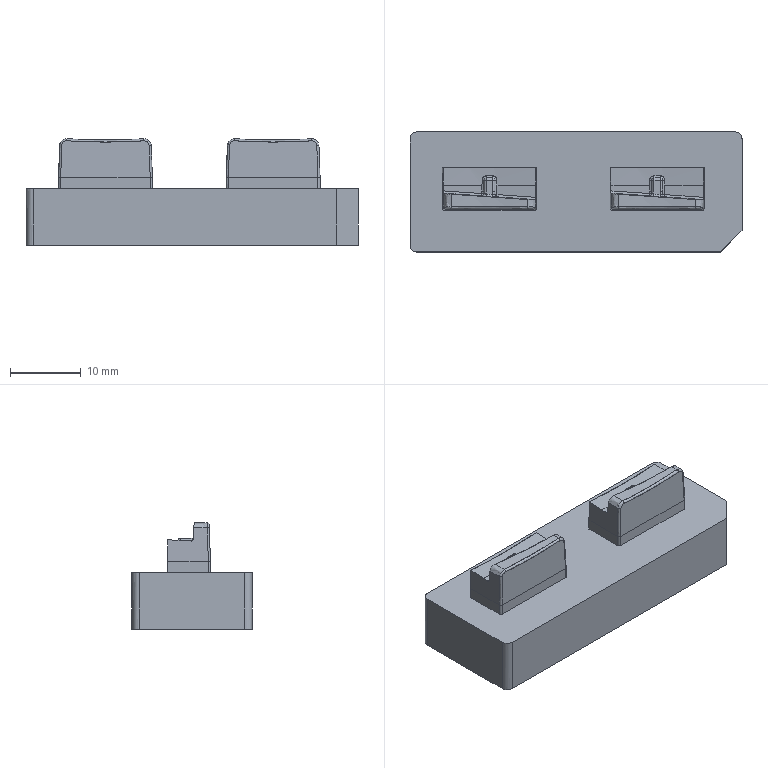NC program | PowerMill | posted with a generic post | part box 47 x 17 x 15.061 mm
Lines 9409 to 10596 of 212044:
N9506 M6
N9507 S22000 M03
N9508 G00 G90 X0.0 Y0.0
N9509 G43 Z9.8009 H27
N9510
N9511 G05 P10000 R4
N9512 X-17.8429 Y1.3228
N9513 Z-1.5208
N9514 G01 Z-2.7208 F1200.0
N9515 X-17.853 Y1.3321 F2000.0
N9516 G03 X-18.0279 Y1.3244 I-0.0836 J-0.0913
N9517 G01 X-18.4675 Y0.8444
N9518 X-18.6964 Y0.72
N9519 X-18.9377 Y0.7308
N9520 X-19.1504 Y0.8766
N9521 X-19.4244 Y0.1186
N9522 X-19.4125 Y0.1119
N9523 G03 X-19.244 Y0.1591 I0.0607 J0.1078
N9524 G01 X-19.1789 Y0.2749
N9525 X-19.0846 Y0.3619
N9526 X-18.9377 Y0.4348
N9527 X-18.6964 Y0.4464
N9528 X-17.1589 Y0.2507
N9529 X-17.0443 Y1.2533 Z-2.7704
N9530 X-17.0545 Y1.2625
N9531 G03 X-17.2293 Y1.2544 I-0.0833 J-0.0914
N9532 G01 X-17.9441 Y0.4701
N9533 X-17.9502 Y0.458
N9534 X-17.9544 Y0.4462
N9535 X-17.9553 Y0.4337
N9536 X-17.9552 Y0.4331
N9537 X-17.9528 Y0.4208
N9538 X-17.9472 Y0.4096
N9539 X-17.9469 Y0.4091
N9540 X-17.9385 Y0.3997
N9541 X-17.928 Y0.3929
N9542 X-17.9158 Y0.3871
N9543 X-17.7315 Y0.3546
N9544 X-16.364 Y0.2017
N9545 G00 Z2.8945
N9546 G01 X-10.9304 Y1.1631 F10000.0
N9547 G00 Z-1.3221
N9548 G01 Z-2.5221 F1200.0
N9549 X-10.9441 F2000.0
N9550 G03 X-11.0679 Y1.0394 I-0.0001 J-0.1238
N9551 G01 X-11.0683 Y-0.1703
N9552 X-11.0652 Y-0.1826
N9553 X-11.0609 Y-0.1935
N9554 X-11.054 Y-0.203
N9555 X-11.0535 Y-0.2036
N9556 X-11.0445 Y-0.2111
N9557 X-11.0339 Y-0.2162
N9558 X-11.0218 Y-0.2202
N9559 X-9.6544 Y-0.3157
N9560 G00 Z2.8502
N9561 G01 X-10.8978 Y1.2816 F10000.0
N9562 G00 Z-1.3718
N9563 G01 Z-2.5718 F1200.0
N9564 X-10.9116 F2000.0
N9565 G03 X-11.0349 Y1.1574 I0.0004 J-0.1238
N9566 G01 X-11.0308 Y-0.1714
N9567 X-11.0277 Y-0.1837
N9568 X-11.0234 Y-0.1946
N9569 X-11.0165 Y-0.2041
N9570 X-11.016 Y-0.2046
N9571 X-11.007 Y-0.2121
N9572 X-10.9964 Y-0.2171
N9573 X-10.9844 Y-0.2211
N9574 X-9.6005 Y-0.3189
N9575 G00 Z2.806
N9576 G01 X-10.8784 Y1.3445 F10000.0
N9577 G00 Z-1.4214
N9578 G01 Z-2.6214 F1200.0
N9579 X-10.8922 F2000.0
N9580 G03 X-11.016 Y1.2208 I-0.0001 J-0.1238
N9581 G01 X-11.0173 Y-0.1704
N9582 X-11.0142 Y-0.1827
N9583 X-11.0099 Y-0.1936
N9584 X-11.003 Y-0.2032
N9585 X-11.0025 Y-0.2037
N9586 X-10.9935 Y-0.2112
N9587 X-10.9829 Y-0.2163
N9588 X-10.9708 Y-0.2203
N9589 X-9.5759 Y-0.3182
N9590 G00 Z2.7618
N9591 G01 X-10.865 Y1.3458 F10000.0
N9592 G00 Z-1.4711
N9593 G01 Z-2.6711 F1200.0
N9594 X-10.8787 F2000.0
N9595 G03 X-11.0026 Y1.2222 I-0.0002 J-0.1238
N9596 G01 X-11.004 Y-0.1699
N9597 X-11.0008 Y-0.1823
N9598 X-10.9965 Y-0.1932
N9599 X-10.9896 Y-0.2027
N9600 X-10.9891 Y-0.2032
N9601 X-10.9801 Y-0.2108
N9602 X-10.9695 Y-0.2158
N9603 X-10.9574 Y-0.2198
N9604 X-9.5573 Y-0.3172
N9605 G00 Z2.7176
N9606 G01 X-10.8399 Y1.3485 F10000.0
N9607 G00 Z-1.5208
N9608 G01 Z-2.7208 F1200.0
N9609 X-10.8537 Y1.3487 F2000.0
N9610 G03 X-10.9787 Y1.2262 I-0.0013 J-0.1238
N9611 G01 X-10.9936 Y-0.1681
N9612 X-10.9905 Y-0.1806
N9613 X-10.9862 Y-0.1916
N9614 X-10.9793 Y-0.2013
N9615 X-10.9788 Y-0.2018
N9616 X-10.9698 Y-0.2094
N9617 X-10.9591 Y-0.2145
N9618 X-10.9468 Y-0.2185
N9619 X-9.5456 Y-0.3101
N9620 G00 Z2.851
N9621 G01 X-10.8323 Y1.3719 F10000.0
N9622 G00 Z-1.5704
N9623 G01 Z-2.7704 F1200.0
N9624 X-10.8461 Y1.372 F2000.0
N9625 G03 X-10.9708 Y1.2491 I-0.0009 J-0.1238
N9626 G01 X-10.9813 Y-0.1611
N9627 X-10.9782 Y-0.1736
N9628 X-10.9739 Y-0.1846
N9629 X-10.967 Y-0.1942
N9630 X-10.9665 Y-0.1947
N9631 X-10.9574 Y-0.2023
N9632 X-10.9468 Y-0.2074
N9633 X-10.9346 Y-0.2114
N9634 X-9.5377 Y-0.3032
N9635 G00 Z2.8075
N9636 G01 X-10.7994 Y1.4057 F10000.0
N9637 G00 Z-1.6201
N9638 G01 Z-2.8201 F1200.0
N9639 X-10.8132 Y1.4059 F2000.0
N9640 G03 X-10.9393 Y1.2846 I-0.0024 J-0.1237
N9641 G01 X-10.9672 Y-0.1505
N9642 X-10.9642 Y-0.1631
N9643 X-10.9599 Y-0.1742
N9644 X-10.953 Y-0.184
N9645 X-10.9525 Y-0.1845
N9646 X-10.9434 Y-0.1922
N9647 X-10.9326 Y-0.1973
N9648 X-10.9203 Y-0.2014
N9649 X-9.4731 Y-0.2911
N9650 G00 Z2.8945
N9651 G01 X4.3292 Y0.1566 F10000.0
N9652 G00 Z-1.5208
N9653 G01 Z-2.7208 F1200.0
N9654 X4.3398 Y0.1478 F2000.0
N9655 G03 X4.514 Y0.1639 I0.0791 J0.0952
N9656 G01 X4.7043 Y0.3928
N9657 X4.9455 Y0.4559
N9658 X6.5958 Y0.2474
N9659 X5.9033 Y1.3286
N9660 X5.8931 Y1.3378
N9661 G03 X5.7183 Y1.3285 I-0.0828 J-0.092
N9662 G01 X5.6692 Y1.2739
N9663 X5.2632 Y0.8444
N9664 X5.1868 Y0.7779
N9665 X4.9455 Y0.7101
N9666 X4.7043 Y0.7813
N9667 X4.6104 Y0.902
N9668 G00 Z2.851
N9669 G01 X6.7059 Y1.2679 F10000.0
N9670 G00 Z-1.5704
N9671 G01 Z-2.7704 F1200.0
N9672 X6.6957 Y1.2771 F2000.0
N9673 G03 X6.5209 Y1.2683 I-0.083 J-0.0918
N9674 G01 X5.7985 Y0.4691
N9675 X5.7924 Y0.4572
N9676 X5.7883 Y0.4455
N9677 X5.7874 Y0.4331
N9678 X5.7875 Y0.4324
N9679 X5.7898 Y0.4202
N9680 X5.7953 Y0.4091
N9681 X5.7957 Y0.4085
N9682 X5.8039 Y0.3992
N9683 X5.8142 Y0.3924
N9684 X5.8263 Y0.3865
N9685 X5.9105 Y0.3705
N9686 X7.3961 Y0.1988
N9687 G00 Z2.8945
N9688 G01 X12.8137 Y1.1625 F10000.0
N9689 G00 Z-1.3221
N9690 G01 Z-2.5221 F1200.0
N9691 X12.8 F2000.0
N9692 G03 X12.6762 Y1.0388 I-0.0001 J-0.1238
N9693 G01 X12.6756 Y-0.1703
N9694 X12.6787 Y-0.1826
N9695 X12.683 Y-0.1935
N9696 X12.6899 Y-0.203
N9697 X12.6904 Y-0.2036
N9698 X12.6994 Y-0.2111
N9699 X12.71 Y-0.2161
N9700 X12.7221 Y-0.2202
N9701 X14.0894 Y-0.3153
N9702 G00 Z2.8502
N9703 G01 X12.8461 Y1.283 F10000.0
N9704 G00 Z-1.3718
N9705 G01 Z-2.5718 F1200.0
N9706 X12.8323 Y1.2829 F2000.0
N9707 G03 X12.709 Y1.1588 I0.0004 J-0.1237
N9708 G01 X12.7131 Y-0.1711
N9709 X12.7163 Y-0.1834
N9710 X12.7206 Y-0.1943
N9711 X12.7274 Y-0.2038
N9712 X12.7279 Y-0.2043
N9713 X12.7369 Y-0.2118
N9714 X12.7475 Y-0.2168
N9715 X12.7596 Y-0.2208
N9716 X14.1411 Y-0.3176
N9717 G00 Z2.806
N9718 G01 X12.8654 Y1.3421 F10000.0
N9719 G00 Z-1.4214
N9720 G01 Z-2.6214 F1200.0
N9721 X12.8517 F2000.0
N9722 G03 X12.7278 Y1.2184 I-0.0001 J-0.1238
N9723 G01 X12.7266 Y-0.1705
N9724 X12.7298 Y-0.1829
N9725 X12.7341 Y-0.1939
N9726 X12.741 Y-0.2034
N9727 X12.7415 Y-0.2039
N9728 X12.7505 Y-0.2114
N9729 X12.7611 Y-0.2165
N9730 X12.7733 Y-0.2205
N9731 X14.1606 Y-0.313
N9732 G00 Z2.7618
N9733 G01 X12.882 Y1.3435 F10000.0
N9734 G00 Z-1.4711
N9735 G01 Z-2.6711 F1200.0
N9736 X12.8682 Y1.3433 F2000.0
N9737 G03 X12.7456 Y1.2185 I0.0012 J-0.1237
N9738 G01 X12.7468 Y1.0856
N9739 X12.7402 Y-0.1689
N9740 X12.7433 Y-0.1813
N9741 X12.7476 Y-0.1923
N9742 X12.7545 Y-0.2019
N9743 X12.755 Y-0.2024
N9744 X12.7641 Y-0.21
N9745 X12.7748 Y-0.215
N9746 X12.787 Y-0.219
N9747 X14.1734 Y-0.3086
N9748 G00 Z2.7176
N9749 G01 X12.8994 Y1.3498 F10000.0
N9750 G00 Z-1.5208
N9751 G01 Z-2.7208 F1200.0
N9752 X12.8857 Y1.3497 F2000.0
N9753 G03 X12.7627 Y1.2252 I0.0008 J-0.1237
N9754 G01 X12.7637 Y1.0856
N9755 X12.7503 Y-0.1681
N9756 X12.7534 Y-0.1806
N9757 X12.7577 Y-0.1916
N9758 X12.7645 Y-0.2012
N9759 X12.765 Y-0.2018
N9760 X12.774 Y-0.2094
N9761 X12.7847 Y-0.2145
N9762 X12.7969 Y-0.2185
N9763 X13.0255 Y-0.2345
N9764 X14.1991 Y-0.3103
N9765 G00 Z2.851
N9766 G01 X12.9125 Y1.3702 F10000.0
N9767 G00 Z-1.5704
N9768 G01 Z-2.7704 F1200.0
N9769 X12.8988 Y1.3703 F2000.0
N9770 G03 X12.774 Y1.2475 I-0.001 J-0.1238
N9771 G01 X12.7626 Y-0.1618
N9772 X12.7657 Y-0.1743
N9773 X12.77 Y-0.1854
N9774 X12.7769 Y-0.195
N9775 X12.7774 Y-0.1955
N9776 X12.7865 Y-0.2031
N9777 X12.7972 Y-0.2081
N9778 X12.8095 Y-0.2121
N9779 X14.2037 Y-0.3012
N9780 G00 Z2.8075
N9781 G01 X12.9445 Y1.4055 F10000.0
N9782 G00 Z-1.6201
N9783 G01 Z-2.8201 F1200.0
N9784 X12.9308 Y1.4058 F2000.0
N9785 G03 X12.8046 Y1.2845 I-0.0025 J-0.1237
N9786 G01 X12.7767 Y-0.1507
N9787 X12.7797 Y-0.1633
N9788 X12.784 Y-0.1744
N9789 X12.7909 Y-0.1842
N9790 X12.7913 Y-0.1847
N9791 X12.8005 Y-0.1924
N9792 X12.8112 Y-0.1975
N9793 X12.8235 Y-0.2016
N9794 X14.2773 Y-0.2953
N9795 G00 Z2.851
N9796 G01 X18.5929 Y-0.0413 F10000.0
N9797 G00 Z-1.5704
N9798 G01 Z-2.7704 F1200.0
N9799 X18.5828 Y-0.0319 F2000.0
N9800 G03 X18.4079 Y-0.0378 I-0.0845 J-0.0904
N9801 G01 X18.3304 Y-0.1206
N9802 X18.214 Y-0.1908
N9803 X17.9727 Y-0.2239
N9804 X17.7458 Y-0.1206
N9805 X17.4902 Y0.1221
N9806 X16.9632 Y0.6963
N9807 X15.7018 Y-0.2627
N9808 X15.7014 Y-0.2764
N9809 G03 X15.8215 Y-0.4038 I0.1237 J-0.0037
N9810 G01 X17.7315 Y-0.4598
N9811 X17.9727 Y-0.3921
N9812 X18.214 Y-0.4275
N9813 X18.4345 Y-0.6031
N9814 X18.4581 Y-0.6682
N9815 G00 Z2.8075
N9816 G01 X14.8066 Y-0.1868 F10000.0
N9817 G00 Z-1.6201
N9818 G01 Z-2.8201 F1200.0
N9819 X14.806 Y-0.2005 F2000.0
N9820 G03 X14.9246 Y-0.3292 I0.1237 J-0.005
N9821 G01 X16.7665 Y-0.4041
N9822 X16.9962 Y-0.3993
N9823 X17.0099 Y-0.395
N9824 X17.0219 Y-0.3892
N9825 X17.0318 Y-0.3802
N9826 X17.0322 Y-0.3798
N9827 X17.0392 Y-0.3684
N9828 X17.0427 Y-0.3555
N9829 X17.0428 Y-0.355
N9830 X17.0425 Y-0.3416
N9831 X17.0385 Y-0.3289
N9832 X17.0324 Y-0.3159
N9833 X16.2082 Y0.6031
N9834 X16.0457 Y0.7548
N9835 G00 Z5.6437
N9836 G01 X13.8538 Y-0.1772 F10000.0
N9837 G00 Z-2.7197
N9838 G01 X13.8919 Y0.0388 Z-2.7236 F1200.0
N9839 X14.0569 Y0.3246 Z-2.7293
N9840 X14.3096 Y0.5366 Z-2.7351
N9841 X14.6197 Y0.6495 Z-2.7408
N9842 X14.9496 Z-2.7466
N9843 X15.2596 Y0.5366 Z-2.7523
N9844 X15.5124 Y0.3246 Z-2.7581
N9845 X15.6773 Y0.0388 Z-2.7639
N9846 X15.7346 Y-0.2861 Z-2.7696
N9847 X15.7335 Y-0.2923 Z-2.7697
N9848 X15.3201 Y-0.2844 Z-2.7769
N9849 X14.7862 Y-0.2561 Z-2.7863
N9850 X13.8487 Y-0.2065 Z-2.8027
N9851 X13.8919 Y0.0388 Z-2.807
N9852 X14.0569 Y0.3246 Z-2.8128
N9853 X14.3096 Y0.5366 Z-2.8185
N9854 X14.6197 Y0.6495 Z-2.8243
N9855 X14.9496 Z-2.83
N9856 X15.2596 Y0.5366 Z-2.8358
N9857 X15.5124 Y0.3246 Z-2.8416
N9858 X15.6773 Y0.0388 Z-2.8473
N9859 X15.7346 Y-0.2861 Z-2.8531
N9860 X15.7335 Y-0.2923 Z-2.8532
N9861 X15.3201 Y-0.2844 Z-2.8604
N9862 X14.7862 Y-0.2561 Z-2.8697
N9863 X14.7846 Y-0.2861
N9864 X14.8163 Y0.1739 F2000.0
N9865 G03 X14.8937 Y0.4082 I0.0087 J0.127
N9866 G01 X13.5722 Y1.254
N9867 G03 X13.3028 Y1.1079 I-0.0944 J-0.1475
N9868 G01 X13.2979 Y0.4665
N9869 G03 X13.4842 Y0.2655 I0.2 J-0.0015
N9870 G01 X14.8163 Y0.1739
N9871 X14.7846 Y-0.2861
N9872 X15.319 Y-0.3144
N9873 X16.0774 Y-0.3288
N9874 X16.1238 Y-0.2997
N9875 X16.1156 Y-0.2455
N9876 X16.0039 Y-0.1206
N9877 X15.0778 Y0.8977
N9878 X14.8298 Y1.0856
N9879 X14.4099 Y1.3268
N9880 X14.361 Y1.3848
N9881 X14.3533 Y1.3921
N9882 X14.3443 Y1.3977
N9883 X13.1478 Y1.9692
N9884 X12.8826 Y2.0517
N9885 X12.833 Y2.0399
N9886 X12.8196 Y1.9906
N9887 X12.8696 Y1.8093
N9888 X12.7912 Y-0.1311
N9889 X12.8042 Y-0.1668
N9890 X12.8385 Y-0.1831
N9891 X14.7846 Y-0.2861
N9892 G00 Z5.6388
N9893 G01 X13.5404 Y-0.1549 F10000.0
N9894 G00 Z-2.7694
N9895 G01 X12.8888 Y-0.1203 Z-2.7808 F1200.0
N9896 X12.8699 Y-0.0991 Z-2.7813
N9897 X12.8959 Y0.3287 Z-2.7888
N9898 X12.9403 Y1.0568 Z-2.8015
N9899 X12.9694 Y1.0733 Z-2.8021
N9900 X13.7507 Y0.6692 Z-2.8174
N9901 X13.7587 Y0.6554 Z-2.8177
N9902 X13.816 Y0.3305 Z-2.8235
N9903 X13.7587 Y0.0056 Z-2.8292
N9904 X13.6623 Y-0.1614 Z-2.8326
N9905 X12.8888 Y-0.1203 Z-2.8461
N9906 X12.8699 Y-0.0991 Z-2.8466
N9907 X12.8959 Y0.3287 Z-2.8541
N9908 X12.9403 Y1.0568 Z-2.8668
N9909 X12.9694 Y1.0733 Z-2.8674
N9910 X13.7507 Y0.6692 Z-2.8827
N9911 X13.7587 Y0.6554 Z-2.883
N9912 X13.816 Y0.3305 Z-2.8888
N9913 X13.7587 Y0.0056 Z-2.8945
N9914 X13.6623 Y-0.1614 Z-2.8979
N9915 X12.8888 Y-0.1203 Z-2.9114
N9916 X12.8699 Y-0.0991 Z-2.9119
N9917 X12.8959 Y0.3287 Z-2.9194
N9918 X12.866 Y0.3305
N9919 X13.3659 F2000.0
N9920 X13.3701 Y0.3263
N9921 X13.3743 Y0.3305
N9922 X13.3701 Y0.3347
N9923 X13.3659 Y0.3305
N9924 X12.866
N9925 X12.8399 Y-0.0973
N9926 X12.8525 Y-0.1336
N9927 X12.8872 Y-0.1503
N9928 X14.5953 Y-0.2409
N9929 X15.155 Y-0.2516
N9930 X15.2014 Y-0.2226
N9931 X15.1934 Y-0.1685
N9932 X15.1511 Y-0.1206
N9933 X14.9732 Y0.0707
N9934 X12.9832 Y1.1
N9935 X12.9356 Y1.099
N9936 X12.9103 Y1.0586
N9937 X12.866 Y0.3305
N9938 X13.0254 Y0.1081 Z-2.819
N9939 X12.9687 Y0.1379 Z-2.8202 F1200.0
N9940 X12.9513 Y0.1385 Z-2.8205
N9941 X12.9395 Y0.122 Z-2.8208
N9942 X12.9237 Y-0.051 Z-2.8238
N9943 X12.9427 Y-0.0728 Z-2.8244
N9944 X13.3195 Y-0.0892 Z-2.8309
N9945 X13.3297 Y-0.0515 Z-2.8316
N9946 X12.9687 Y0.1379 Z-2.8387
N9947 X12.9513 Y0.1385 Z-2.839
N9948 X12.9395 Y0.122 Z-2.8394
N9949 X12.9237 Y-0.051 Z-2.8424
N9950 X12.9427 Y-0.0728 Z-2.8429
N9951 X13.3195 Y-0.0892 Z-2.8495
N9952 X13.3297 Y-0.0515 Z-2.8502
N9953 X12.9687 Y0.1379 Z-2.8573
N9954 X12.9513 Y0.1385 Z-2.8576
N9955 X12.9395 Y0.122 Z-2.858
N9956 X12.9237 Y-0.051 Z-2.861
N9957 X12.9427 Y-0.0728 Z-2.8615
N9958 X13.3195 Y-0.0892 Z-2.8681
N9959 X13.3297 Y-0.0515 Z-2.8688
N9960 X12.9687 Y0.1379 Z-2.8759
N9961 X12.9513 Y0.1385 Z-2.8762
N9962 X12.9395 Y0.122 Z-2.8765
N9963 X12.9237 Y-0.051 Z-2.8796
N9964 X12.9427 Y-0.0728 Z-2.8801
N9965 X13.3195 Y-0.0892 Z-2.8867
N9966 X13.3297 Y-0.0515 Z-2.8873
N9967 X12.9687 Y0.1379 Z-2.8944
N9968 X12.9513 Y0.1385 Z-2.8948
N9969 X12.9395 Y0.122 Z-2.8951
N9970 X12.9237 Y-0.051 Z-2.8981
N9971 X12.9427 Y-0.0728 Z-2.8986
N9972 X13.3195 Y-0.0892 Z-2.9052
N9973 X13.3297 Y-0.0515 Z-2.9059
N9974 X12.9687 Y0.1379 Z-2.913
N9975 X12.9513 Y0.1385 Z-2.9133
N9976 X12.9395 Y0.122 Z-2.9137
N9977 X12.9237 Y-0.051 Z-2.9167
N9978 X12.9427 Y-0.0728 Z-2.9172
N9979 X13.3195 Y-0.0892 Z-2.9238
N9980 X13.3297 Y-0.0515 Z-2.9245
N9981 X12.9687 Y0.1379 Z-2.9316
N9982 X12.9513 Y0.1385 Z-2.9319
N9983 X12.9395 Y0.122 Z-2.9322
N9984 X12.9237 Y-0.051 Z-2.9353
N9985 X12.9427 Y-0.0728 Z-2.9358
N9986 X13.3195 Y-0.0892 Z-2.9424
N9987 X13.3297 Y-0.0515 Z-2.943
N9988 X12.9687 Y0.1379 Z-2.9502
N9989 X12.9513 Y0.1385 Z-2.9505
N9990 X12.9395 Y0.122 Z-2.9508
N9991 X12.9237 Y-0.051 Z-2.9539
N9992 X12.9427 Y-0.0728 Z-2.9544
N9993 X13.3195 Y-0.0892 Z-2.9609
N9994 X13.3297 Y-0.0515 Z-2.9616
N9995 X12.9687 Y0.1379 Z-2.9687
N9996 X12.9513 Y0.1385 Z-2.969
N9997 X12.9391 Y0.1659
N9998 X12.9188 Y0.1493 F2000.0
N9999 X12.9097 Y0.1248
N10000 X12.8938 Y-0.0482
N10001 X12.9059 Y-0.0857
N10002 X12.9414 Y-0.1028
N10003 X13.3182 Y-0.1192
N10004 X13.3687 Y-0.0822
N10005 X13.3436 Y-0.0249
N10006 X12.9827 Y0.1645
N10007 X12.9611 Y0.1702
N10008 X12.9391 Y0.1659
N10009 G00 Z2.7207
N10010 G01 X8.5418 Y0.2113 F10000.0
N10011 G00 Z-1.3221
N10012 G01 Z-2.5221 F1200.0
N10013 X8.5408 Y0.1976 F2000.0
N10014 G03 X8.6555 Y0.0654 I0.1234 J-0.0088
N10015 G01 X10.2462 Y-0.0475
N10016 X10.2598 Y-0.0447
N10017 X10.2719 Y-0.0404
N10018 X10.2824 Y-0.033
N10019 X10.2829 Y-0.0325
N10020 X10.291 Y-0.0226
N10021 X10.296 Y-0.0108
N10022 X10.2997 Y0.0026
N10023 X10.2939 Y1.4164
N10024 G00 Z2.8502
N10025 G01 X8.4998 Y0.2195 F10000.0
N10026 G00 Z-1.3718
N10027 G01 Z-2.5718 F1200.0
N10028 X8.4988 Y0.2058 F2000.0
N10029 G03 X8.6132 Y0.0734 I0.1234 J-0.009
N10030 G01 X10.2086 Y-0.043
N10031 X10.2222 Y-0.0402
N10032 X10.2343 Y-0.036
N10033 X10.2448 Y-0.0286
N10034 X10.2453 Y-0.0282
N10035 X10.2534 Y-0.0182
N10036 X10.2585 Y-0.0065
N10037 X10.2623 Y0.0069
N10038 X10.2619 Y1.5318
N10039 G00 Z2.806
N10040 G01 X8.4744 Y0.2258 F10000.0
N10041 G00 Z-1.4214
N10042 G01 Z-2.6214 F1200.0
N10043 X8.4734 Y0.2121 F2000.0
N10044 G03 X8.5876 Y0.0795 I0.1234 J-0.0092
N10045 G01 X10.1952 Y-0.0402
N10046 X10.2088 Y-0.0375
N10047 X10.2209 Y-0.0332
N10048 X10.2315 Y-0.0258
N10049 X10.2319 Y-0.0254
N10050 X10.2401 Y-0.0154
N10051 X10.2452 Y-0.0036
N10052 X10.2489 Y0.0097
N10053 X10.2449 Y1.5681
N10054 X10.2461 Y1.5952
N10055 G00 Z2.7618
N10056 G01 X8.4548 Y0.2282 F10000.0
N10057 G00 Z-1.4711
N10058 G01 Z-2.6711 F1200.0
N10059 X8.4537 Y0.2145 F2000.0
N10060 G03 X8.5669 Y0.081 I0.1233 J-0.0102
N10061 G01 X9.3808 Y0.0186
N10062 X10.1953 Y-0.035
N10063 X10.2074 Y-0.0307
N10064 X10.2179 Y-0.0232
N10065 X10.2184 Y-0.0228
N10066 X10.2265 Y-0.0128
N10067 X10.2316 Y-0.001
N10068 X10.2353 Y0.0123
N10069 X10.2278 Y1.5681
N10070 X10.2296 Y1.6063
N10071 G00 Z2.8945
N10072 G01 X8.4484 Y0.2381 F10000.0
N10073 G00 Z-1.5208
N10074 G01 Z-2.7208 F1200.0
N10075 X8.4473 Y0.2244 F2000.0
N10076 G03 X8.561 Y0.0914 I0.1234 J-0.0096
N10077 G01 X10.1696 Y-0.0348
N10078 X10.1833 Y-0.032
N10079 X10.1956 Y-0.0277
N10080 X10.2061 Y-0.0203
N10081 X10.2066 Y-0.0199
N10082 X10.2148 Y-0.0098
N10083 X10.2199 Y0.0021
N10084 X10.2236 Y0.0156
N10085 X10.2088 Y1.5681
N10086 X10.2104 Y1.6046
N10087 G00 Z2.851
N10088 G01 X8.3713 Y0.253 F10000.0
N10089 G00 Z-1.5704
N10090 G01 Z-2.7704 F1200.0
N10091 X8.3702 Y0.2393 F2000.0
N10092 G03 X8.484 Y0.1063 I0.1234 J-0.0097
N10093 G01 X10.1554 Y-0.0243
N10094 X10.1691 Y-0.0215
N10095 X10.1814 Y-0.0172
N10096 X10.192 Y-0.0097
N10097 X10.1924 Y-0.0093
N10098 X10.2006 Y0.0008
N10099 X10.2057 Y0.0127
N10100 X10.2093 Y0.0262
N10101 X10.1898 Y1.5681
N10102 X10.1933 Y1.6561
N10103 X9.3035 Y2.2713 Z-2.8201
N10104 X9.3158 Y2.1344
N10105 G02 X8.682 Y2.2336 I-0.1183 J1.3186
N10106 G01 X8.5962 Y2.2735
N10107 X8.5642 Y2.2636
N10108 X8.2159 Y2.0506
N10109 X8.0966 Y2.0078
N10110 X8.0768 Y1.9947
N10111 X8.0153 Y1.9625
N10112 X7.3671 Y1.2524
N10113 X7.6834 Y0.9117
N10114 X8.3172 Y1.5
N10115 X8.3409 Y1.5188
N10116 X8.5699 Y1.651
N10117 X8.6196 Y1.6712
N10118 X8.6729 Y1.6775
N10119 X8.8571 Y1.6746
N10120 X8.8446 Y1.2139
N10121 X9.1221 Y1.2064
N10122 X9.1699 Y1.1845
N10123 X9.1871 Y1.1349
N10124 X9.1835 Y1.0821
N10125 X9.1628 Y1.0399
N10126 X9.1186 Y1.0243
N10127 X8.8193 Y1.039
N10128 G02 X8.7809 Y1.1906 I0.004 J0.0817
N10129 G01 X8.8 Y1.2021
N10130 X8.8214 Y1.2112
N10131 X8.8446 Y1.2139
N10132 X8.8571 Y1.6746
N10133 X9.2241 Y1.6689
N10134 X9.4927 Y1.6808
N10135 G02 X9.7022 Y1.4828 I0.0095 J-0.1998
N10136 G01 X9.709 Y0.7242
N10137 G02 X9.4932 Y0.523 I-0.2 J-0.0018
N10138 G01 X7.7708 Y0.6601
N10139 G02 X7.6834 Y0.9117 I0.0115 J0.145
N10140 G01 X7.3671 Y1.2524
N10141 X6.6024 Y0.4145
N10142 X6.5962 Y0.4022
N10143 X6.5921 Y0.39
N10144 X6.5914 Y0.3772
N10145 Y0.3765
N10146 X6.5942 Y0.364
N10147 X6.6003 Y0.3527
N10148 X6.6007 Y0.3522
N10149 X6.6096 Y0.343
N10150 X6.6207 Y0.3365
N10151 X6.6335 Y0.3312
N10152 X7.8404 Y0.1875
N10153 X10.142 Y-0.011
N10154 X10.1558 Y-0.0083
N10155 X10.1681 Y-0.004
N10156 X10.1788 Y0.0035
N10157 X10.1793 Y0.0039
N10158 X10.1875 Y0.014
N10159 X10.1926 Y0.026
N10160 X10.1963 Y0.0396
N10161 X10.1837 Y0.9246
N10162 X10.1613 Y1.8093
N10163 X10.2315 Y2.0506
N10164 X10.3955 Y2.2918
N10165 X10.4584 Y2.3515
N10166 X9.6381 Y1.8419 Z-2.7197
N10167 X9.6569 Y1.8512 Z-2.7201 F1200.0
N10168 X9.7036 Y1.7705 Z-2.7217
N10169 X9.7608 Y1.4456 Z-2.7275
N10170 X9.7036 Y1.1207 Z-2.7332
N10171 X9.5386 Y0.8349 Z-2.739
N10172 X9.2859 Y0.6229 Z-2.7448
N10173 X8.9758 Y0.51 Z-2.7505
N10174 X8.6459 Z-2.7563
N10175 X8.3358 Y0.6229 Z-2.762
N10176 X8.0831 Y0.8349 Z-2.7678
N10177 X8.0087 Y0.9638 Z-2.7704
N10178 X8.0352 Y0.9924 Z-2.7711
N10179 X8.8251 Y1.4192 Z-2.7867
N10180 X9.3017 Y1.6767 Z-2.7962
N10181 X9.6569 Y1.8512 Z-2.8031
N10182 X9.7036 Y1.7705 Z-2.8047
N10183 X9.7608 Y1.4456 Z-2.8105
N10184 X9.7036 Y1.1207 Z-2.8162
N10185 X9.5386 Y0.8349 Z-2.822
N10186 X9.2859 Y0.6229 Z-2.8278
N10187 X8.9758 Y0.51 Z-2.8335
N10188 X8.6459 Z-2.8393
N10189 X8.3358 Y0.6229 Z-2.845
N10190 X8.0831 Y0.8349 Z-2.8508
N10191 X8.0087 Y0.9638 Z-2.8534
N10192 X8.0352 Y0.9924 Z-2.8541
N10193 X8.8251 Y1.4192 Z-2.8697
N10194 X8.8109 Y1.4456
N10195 X9.0297 Y1.0371 F2000.0
N10196 X8.6334 Y0.8249
N10197 G03 X8.6767 Y0.616 I0.0525 J-0.0981
N10198 G01 X9.4608 Y0.5507
N10199 G03 X9.6774 Y0.7524 I0.0166 J0.1993
N10200 G01 X9.6732 Y1.1033
N10201 G03 X9.4259 Y1.2494 I-0.168 J-0.002
N10202 G01 X9.0297 Y1.0371
N10203 X8.8109 Y1.4456
N10204 X8.0166 Y1.0164
N10205 X7.4124 Y0.366
N10206 X7.4017 Y0.3157
N10207 X7.441 Y0.2826
N10208 X7.5992 Y0.2569
N10209 X10.1224 Y0.0136
N10210 X10.1616 Y0.0271
N10211 X10.1772 Y0.0655
N10212 X10.1747 Y0.1206
N10213 X10.1058 Y1.8093
N10214 X10.1685 Y2.0506
N10215 X10.1758 Y2.0644
N10216 X10.1665 Y2.1236
N10217 X10.107 Y2.1313
N10218 X9.7704 Y1.9404
N10219 X9.2879 Y1.7034
N10220 X8.8109 Y1.4456
N10221 X9.2649 Y0.6947 Z-2.7694
N10222 X9.2112 Y0.6671 Z-2.7704 F1200.0
N10223 X8.4738 Y0.2878 Z-2.7849
N10224 X8.4803 Y0.2502 Z-2.7856
N10225 X9.05 Y0.1735 Z-2.7956
N10226 X9.9327 Y0.0961 Z-2.8111
N10227 X10.0802 Y0.3516 Z-2.8162
N10228 X10.04 Y1.0617 Z-2.8286
N10229 X10.0108 Y1.0783 Z-2.8292
N10230 X9.2112 Y0.6671 Z-2.8449
N10231 X8.4738 Y0.2878 Z-2.8594
N10232 X8.4803 Y0.2502 Z-2.8601
N10233 X9.05 Y0.1735 Z-2.8701
N10234 X9.9327 Y0.0961 Z-2.8856
N10235 X10.0802 Y0.3516 Z-2.8907
N10236 X10.04 Y1.0617 Z-2.9031
N10237 X10.0108 Y1.0783 Z-2.9037
N10238 X9.2112 Y0.6671 Z-2.9194
N10239 X9.1975 Y0.6938
N10240 X8.4601 Y0.3145 F2000.0
N10241 G03 X8.4763 Y0.2205 I0.0228 J-0.0445
N10242 G01 X9.0467 Y0.1437
N10243 X10.07 Y0.0539
N10244 X10.1093 Y0.068
N10245 X10.1243 Y0.107
N10246 X10.1234 Y0.1206
N10247 X10.0699 Y1.0634
N10248 X10.0448 Y1.1039
N10249 X9.9971 Y1.105
N10250 X9.1975 Y0.6938
N10251 G00 Z2.851
N10252 G01 X-5.1622 Y-0.0004 F10000.0
N10253 G00 Z-1.5704
N10254 G01 Z-2.7704 F1200.0
N10255 X-5.1734 Y0.0076 F2000.0
N10256 G03 X-5.346 Y-0.0209 I-0.072 J-0.1006
N10257 G01 X-5.428 Y-0.1353
N10258 X-5.6692 Y-0.2247
N10259 X-5.9105 Y-0.1877
N10260 X-6.0156 Y-0.1206
N10261 X-6.7796 Y0.6989
N10262 X-8.0198 Y-0.2494
N10263 X-8.0203 Y-0.2632
N10264 G03 X-7.9017 Y-0.3918 I0.1236 J-0.005
N10265 G01 X-6.1278 Y-0.4633
N10266 X-5.6692 Y-0.3917
N10267 X-5.428 Y-0.4841
N10268 X-5.3092 Y-0.6031
N10269 X-5.2877 Y-0.6627
N10270 G00 Z2.8075
N10271 G01 X-8.9278 Y-0.1871 F10000.0
N10272 G00 Z-1.6201
N10273 G01 Z-2.8201 F1200.0
N10274 X-8.9287 Y-0.2008 F2000.0
N10275 G03 X-8.8128 Y-0.332 I0.1235 J-0.0077
N10276 G01 X-8.8054 Y-0.3324
N10277 X-6.7569 Y-0.3935
N10278 X-6.7427 Y-0.3897
N10279 X-6.7302 Y-0.3843
N10280 X-6.7197 Y-0.3755
N10281 X-6.7193 Y-0.3751
N10282 X-6.7119 Y-0.3636
N10283 X-6.708 Y-0.3505
N10284 X-6.7079 Y-0.35
N10285 X-6.708 Y-0.3363
N10286 X-6.712 Y-0.3232
N10287 X-6.7183 Y-0.31
N10288 X-7.6895 Y0.7613
N10289 G00 Z5.6396
N10290 G01 X-9.8977 Y-0.1589 F10000.0
N10291 G00 Z-2.7197
N10292 G01 X-9.8616 Y0.0458 Z-2.7234 F1200.0
N10293 X-9.6967 Y0.3315 Z-2.7291
N10294 X-9.4439 Y0.5436 Z-2.7349
N10295 X-9.1339 Y0.6564 Z-2.7406
N10296 X-8.8039 Z-2.7464
N10297 X-8.4939 Y0.5436 Z-2.7521
N10298 X-8.2412 Y0.3315 Z-2.7579
N10299 X-8.0762 Y0.0458 Z-2.7637
N10300 X-8.0189 Y-0.2792 Z-2.7694
N10301 X-8.0197 Y-0.2838 Z-2.7695
N10302 X-8.9678 Y-0.2492 Z-2.7861
N10303 X-9.769 Y-0.2199 Z-2.8
N10304 X-9.907 Y-0.2118 Z-2.8025
N10305 X-9.8616 Y0.0458 Z-2.807
N10306 X-9.6967 Y0.3315 Z-2.8128
N10307 X-9.4439 Y0.5436 Z-2.8185
N10308 X-9.1339 Y0.6564 Z-2.8243
N10309 X-8.8039 Z-2.8301
N10310 X-8.4939 Y0.5436 Z-2.8358
N10311 X-8.2412 Y0.3315 Z-2.8416
N10312 X-8.0762 Y0.0458 Z-2.8473
N10313 X-8.0189 Y-0.2792 Z-2.8531
N10314 X-8.0197 Y-0.2838 Z-2.8532
N10315 X-8.9678 Y-0.2492 Z-2.8697
N10316 X-8.9689 Y-0.2792
N10317 X-8.9403 Y0.1787 F2000.0
N10318 G03 X-8.8585 Y0.4146 I0.0081 J0.1293
N10319 G01 X-9.1506 Y0.6163
N10320 X-10.1733 Y1.2613
N10321 G03 X-10.4409 Y1.1149 I-0.0931 J-0.1476
N10322 G01 X-10.4453 Y0.4621
N10323 G03 X-10.2577 Y0.2611 I0.2 J-0.0014
N10324 G01 X-8.9403 Y0.1787
N10325 X-8.9689 Y-0.2792
N10326 X-7.6658 Y-0.3268
N10327 G03 X-7.6262 Y-0.2441 I0.0018 J0.05
N10328 G01 X-7.7331 Y-0.1206
N10329 X-8.8054 Y1.0441
N10330 X-9.3697 Y1.3268
N10331 X-9.5292 Y1.4636
N10332 X-10.4941 Y1.9293
N10333 X-10.86 Y2.0497
N10334 X-10.9102 Y2.0384
N10335 X-10.9239 Y1.9889
N10336 X-10.8743 Y1.8093
N10337 X-10.9527 Y-0.1313
N10338 X-10.9398 Y-0.1669
N10339 X-10.9057 Y-0.1832
N10340 X-9.7704 Y-0.2499
N10341 X-8.9689 Y-0.2792
N10342 G00 Z5.6395
N10343 G01 X-10.2085 Y-0.1586 F10000.0
N10344 G00 Z-2.7694
N10345 G01 X-10.8553 Y-0.1205 Z-2.7807 F1200.0
N10346 X-10.8741 Y-0.0993 Z-2.7812
N10347 X-10.8481 Y0.3269 Z-2.7886
N10348 X-10.8036 Y1.0567 Z-2.8014
N10349 X-10.7744 Y1.0733 Z-2.802
N10350 X-9.9948 Y0.6701 Z-2.8173
N10351 X-9.9853 Y0.6537 Z-2.8176
N10352 X-9.928 Y0.3288 Z-2.8234
N10353 X-9.9853 Y0.0038 Z-2.8292
N10354 X-10.0833 Y-0.1659 Z-2.8326
N10355 X-10.8553 Y-0.1205 Z-2.8461
N10356 X-10.8741 Y-0.0993 Z-2.8466
N10357 X-10.8481 Y0.3269 Z-2.854
N10358 X-10.8036 Y1.0567 Z-2.8668
N10359 X-10.7744 Y1.0733 Z-2.8674
N10360 X-9.9948 Y0.6701 Z-2.8827
N10361 X-9.9853 Y0.6537 Z-2.883
N10362 X-9.928 Y0.3288 Z-2.8888
N10363 X-9.9853 Y0.0038 Z-2.8945
N10364 X-10.0833 Y-0.1659 Z-2.8979
N10365 X-10.8553 Y-0.1205 Z-2.9114
N10366 X-10.8741 Y-0.0993 Z-2.9119
N10367 X-10.8481 Y0.3269 Z-2.9194
N10368 X-10.878 Y0.3288
N10369 X-10.3773 F2000.0
N10370 X-10.3728 Y0.3243
N10371 X-10.3683 Y0.3288
N10372 X-10.3728 Y0.3332
N10373 X-10.3773 Y0.3288
N10374 X-10.878
N10375 X-10.904 Y-0.0975
N10376 X-10.8915 Y-0.1337
N10377 X-10.857 Y-0.1505
N10378 X-10.0116 Y-0.2002
N10379 X-8.5903 Y-0.2497
N10380 X-8.5433 Y-0.221
N10381 X-8.5511 Y-0.1665
N10382 X-8.5919 Y-0.1206
N10383 X-8.8054 Y0.0888
N10384 X-10.7606 Y1.0999
N10385 X-10.8083 Y1.099
N10386 X-10.8335 Y1.0586
N10387 X-10.878 Y0.3288
N10388 X-10.8075 Y0.1335 Z-2.819
N10389 X-10.8118 Y0.1284 Z-2.8192 F1200.0
N10390 X-10.8131 Y0.1223 Z-2.8193
N10391 X-10.8222 Y-0.0506 Z-2.8223
N10392 X-10.8032 Y-0.0716 Z-2.8228
N10393 X-10.4254 Y-0.0888 Z-2.8294
N10394 X-10.4152 Y-0.0511 Z-2.8301
N10395 X-10.7829 Y0.1419 Z-2.8373
N10396 X-10.7999 Y0.1427 Z-2.8376
N10397 X-10.8118 Y0.1284 Z-2.8379
N10398 X-10.8131 Y0.1223 Z-2.838
N10399 X-10.8222 Y-0.0506 Z-2.8411
N10400 X-10.8032 Y-0.0716 Z-2.8416
N10401 X-10.4254 Y-0.0888 Z-2.8482
N10402 X-10.4152 Y-0.0511 Z-2.8488
N10403 X-10.7829 Y0.1419 Z-2.8561
N10404 X-10.7999 Y0.1427 Z-2.8564
N10405 X-10.8118 Y0.1284 Z-2.8567
N10406 X-10.8131 Y0.1223 Z-2.8568
N10407 X-10.8222 Y-0.0506 Z-2.8598
N10408 X-10.8032 Y-0.0716 Z-2.8603
N10409 X-10.4254 Y-0.0888 Z-2.8669
N10410 X-10.4152 Y-0.0511 Z-2.8676
N10411 X-10.7829 Y0.1419 Z-2.8749
N10412 X-10.7999 Y0.1427 Z-2.8752
N10413 X-10.8118 Y0.1284 Z-2.8755
N10414 X-10.8131 Y0.1223 Z-2.8756
N10415 X-10.8222 Y-0.0506 Z-2.8786
N10416 X-10.8032 Y-0.0716 Z-2.8791
N10417 X-10.4254 Y-0.0888 Z-2.8857
N10418 X-10.4152 Y-0.0511 Z-2.8864
N10419 X-10.7829 Y0.1419 Z-2.8936
N10420 X-10.7999 Y0.1427 Z-2.8939
N10421 X-10.8118 Y0.1284 Z-2.8943
N10422 X-10.8131 Y0.1223 Z-2.8944
N10423 X-10.8222 Y-0.0506 Z-2.8974
N10424 X-10.8032 Y-0.0716 Z-2.8979
N10425 X-10.4254 Y-0.0888 Z-2.9045
N10426 X-10.4152 Y-0.0511 Z-2.9052
N10427 X-10.7829 Y0.1419 Z-2.9124
N10428 X-10.7999 Y0.1427 Z-2.9127
N10429 X-10.8118 Y0.1284 Z-2.913
N10430 X-10.8131 Y0.1223 Z-2.9131
N10431 X-10.8222 Y-0.0506 Z-2.9162
N10432 X-10.8032 Y-0.0716 Z-2.9167
N10433 X-10.4254 Y-0.0888 Z-2.9233
N10434 X-10.4152 Y-0.0511 Z-2.9239
N10435 X-10.7829 Y0.1419 Z-2.9312
N10436 X-10.7999 Y0.1427 Z-2.9315
N10437 X-10.8118 Y0.1284 Z-2.9318
N10438 X-10.8131 Y0.1223 Z-2.9319
N10439 X-10.8222 Y-0.0506 Z-2.9349
N10440 X-10.8032 Y-0.0716 Z-2.9354
N10441 X-10.4254 Y-0.0888 Z-2.942
N10442 X-10.4152 Y-0.0511 Z-2.9427
N10443 X-10.7829 Y0.1419 Z-2.95
N10444 X-10.7999 Y0.1427 Z-2.9503
N10445 X-10.8118 Y0.1284 Z-2.9506
N10446 X-10.8131 Y0.1223 Z-2.9507
N10447 X-10.8222 Y-0.0506 Z-2.9537
N10448 X-10.8032 Y-0.0716 Z-2.9542
N10449 X-10.4254 Y-0.0888 Z-2.9608
N10450 X-10.4152 Y-0.0511 Z-2.9615
N10451 X-10.7829 Y0.1419 Z-2.9687
N10452 X-10.7999 Y0.1427 Z-2.969
N10453 X-10.8115 Y0.1703
N10454 X-10.8307 Y0.1562 F2000.0
N10455 X-10.8411 Y0.1348
N10456 X-10.8429 Y0.1263
N10457 X-10.8522 Y-0.049
N10458 X-10.8393 Y-0.0852
N10459 X-10.8045 Y-0.1016
N10460 X-10.4267 Y-0.1187
N10461 X-10.3762 Y-0.0818
N10462 X-10.4012 Y-0.0245
N10463 X-10.769 Y0.1685
N10464 X-10.7901 Y0.1742
N10465 X-10.8115 Y0.1703
N10466 G00 Z2.7207
N10467 G01 X-15.2014 Y0.2117 F10000.0
N10468 G00 Z-1.3221
N10469 G01 Z-2.5221 F1200.0
N10470 X-15.2024 Y0.198 F2000.0
N10471 G03 X-15.0878 Y0.0658 I0.1234 J-0.0088
N10472 G01 X-13.4975 Y-0.0475
N10473 X-13.484 Y-0.0447
N10474 X-13.4719 Y-0.0404
N10475 X-13.4614 Y-0.033
N10476 X-13.4609 Y-0.0326
N10477 X-13.4528 Y-0.0227
N10478 X-13.4477 Y-0.0109
N10479 X-13.444 Y0.0024
N10480 X-13.4443 Y1.4225
N10481 G00 Z2.8502
N10482 G01 X-15.2435 Y0.2198 F10000.0
N10483 G00 Z-1.3718
N10484 G01 Z-2.5718 F1200.0
N10485 X-15.2446 Y0.2061 F2000.0
N10486 G03 X-15.1302 Y0.0737 I0.1235 J-0.009
N10487 G01 X-13.5356 Y-0.043
N10488 X-13.522 Y-0.0402
N10489 X-13.5099 Y-0.036
N10490 X-13.4994 Y-0.0286
N10491 X-13.4989 Y-0.0281
N10492 X-13.4908 Y-0.0182
N10493 X-13.4857 Y-0.0064
N10494 X-13.4819 Y0.0069
N10495 X-13.4823 Y1.5315
N10496 G00 Z2.806
N10497 G01 X-15.2676 Y0.2266 F10000.0
N10498 G00 Z-1.4214
N10499 G01 Z-2.6214 F1200.0
N10500 X-15.2686 Y0.2129 F2000.0
N10501 G03 X-15.1545 Y0.0802 I0.1234 J-0.0093
N10502 G01 X-13.5491 Y-0.0402
N10503 X-13.5355 Y-0.0375
N10504 X-13.5234 Y-0.0332
N10505 X-13.5129 Y-0.0259
N10506 X-13.5124 Y-0.0255
N10507 X-13.5043 Y-0.0156
N10508 X-13.4991 Y-0.0038
N10509 X-13.4954 Y0.0095
N10510 X-13.4893 Y1.6125
N10511 G00 Z2.7618
N10512 G01 X-15.2704 Y0.2294 F10000.0
N10513 G00 Z-1.4711
N10514 G01 Z-2.6711 F1200.0
N10515 X-15.2715 Y0.2157 F2000.0
N10516 G03 X-15.1574 Y0.083 I0.1234 J-0.0093
N10517 G01 X-13.5619 Y-0.0375
N10518 X-13.5484 Y-0.0348
N10519 X-13.5362 Y-0.0306
N10520 X-13.5257 Y-0.0232
N10521 X-13.5252 Y-0.0228
N10522 X-13.5171 Y-0.0128
N10523 X-13.5119 Y-0.0011
N10524 X-13.5082 Y0.0122
N10525 X-13.5053 Y1.6079
N10526 G00 Z2.7176
N10527 G01 X-15.2862 Y0.2359 F10000.0
N10528 G00 Z-1.5208
N10529 G01 Z-2.7208 F1200.0
N10530 X-15.2872 Y0.2222 F2000.0
N10531 G03 X-15.1734 Y0.0892 I0.1233 J-0.0096
N10532 G01 X-13.5747 Y-0.0348
N10533 X-13.561 Y-0.032
N10534 X-13.5488 Y-0.0277
N10535 X-13.5382 Y-0.0203
N10536 X-13.5377 Y-0.0199
N10537 X-13.5296 Y-0.0098
N10538 X-13.5245 Y0.0021
N10539 X-13.5208 Y0.0156
N10540 X-13.5359 Y1.5681
N10541 X-13.5356 Y1.5746
N10542 G00 Z2.851
N10543 G01 X-15.3034 Y0.2465 F10000.0
N10544 G00 Z-1.5704
N10545 G01 Z-2.7704 F1200.0
N10546 X-15.3045 Y0.2328 F2000.0
N10547 G03 X-15.1907 Y0.0998 I0.1234 J-0.0096
N10548 G01 X-13.5877 Y-0.0243
N10549 X-13.574 Y-0.0216
N10550 X-13.5618 Y-0.0173
N10551 X-13.5512 Y-0.0098
N10552 X-13.5507 Y-0.0094
N10553 X-13.5426 Y0.0007
N10554 X-13.5375 Y0.0127
N10555 X-13.5339 Y0.0262
N10556 X-13.5542 Y1.5681
N10557 X-13.5534 Y1.5896
N10558 G00 Z2.8075
N10559 G01 X-15.3412 Y0.2779 F10000.0
N10560 G00 Z-1.6201
N10561 G01 Z-2.8201 F1200.0
N10562 X-15.3424 Y0.2642 F2000.0
N10563 G03 X-15.2298 Y0.1302 I0.1233 J-0.0107
N10564 G01 X-13.6021 Y-0.0109
N10565 X-13.5883 Y-0.0082
N10566 X-13.5759 Y-0.0039
N10567 X-13.5652 Y0.0036
N10568 X-13.5647 Y0.004
N10569 X-13.5565 Y0.0142
N10570 X-13.5514 Y0.0262
N10571 X-13.5478 Y0.0399
N10572 X-13.5791 Y1.6318
N10573 G00 Z1.3799
N10574 G01 X-16.2497 Y1.19 F10000.0
N10575 G00 Z-1.6201
N10576 G01 Z-2.8201 F1200.0
N10577 X-16.2599 Y1.1993 F2000.0
N10578 G03 X-16.4347 Y1.1911 I-0.0833 J-0.0915
N10579 G01 X-17.1417 Y0.4144
N10580 X-17.1479 Y0.4021
N10581 X-17.1521 Y0.3899
N10582 X-17.1528 Y0.3771
N10583 X-17.1527 Y0.3765
N10584 X-17.1499 Y0.364
N10585 X-17.1439 Y0.3527
N10586 X-17.1435 Y0.3522
N10587 X-17.1346 Y0.343
N10588 X-17.1236 Y0.3365
N10589 X-17.1108 Y0.3311
N10590 X-16.0428 Y0.2007
N10591 X-15.5734 Y0.16
N10592 G00 Z3.1728
N10593 G01 X-14.1371 Y1.9057 F10000.0
N10594 G00 Z-2.7197
N10595 G01 X-14.0742 Y1.7968 Z-2.7219 F1200.0
N10596 X-14.0169 Y1.4719 Z-2.7277
N10597 X-14.0742 Y1.1469 Z-2.7334
N10598 X-14.2391 Y0.8612 Z-2.7392
N10599 X-14.4919 Y0.6491 Z-2.745
N10600 X-14.8019 Y0.5363 Z-2.7507
N10601 X-15.1318 Z-2.7565
N10602 X-15.4419 Y0.6491 Z-2.7622
N10603 X-15.6946 Y0.8612 Z-2.768
N10604 X-15.7507 Y0.9584 Z-2.7699
N10605 X-14.9513 Y1.4463 Z-2.7863
N10606 X-14.153 Y1.9333 Z-2.8026
N10607 X-14.0742 Y1.7968 Z-2.8054
N10608 X-14.0169 Y1.4719 Z-2.8111
N10609 X-14.0742 Y1.1469 Z-2.8169
N10610 X-14.2391 Y0.8612 Z-2.8226
N10611 X-14.4919 Y0.6491 Z-2.8284
N10612 X-14.8019 Y0.5363 Z-2.8342
N10613 X-15.1318 Z-2.8399
N10614 X-15.4419 Y0.6491 Z-2.8457
N10615 X-15.6946 Y0.8612 Z-2.8514
N10616 X-15.7507 Y0.9584 Z-2.8534
N10617 X-14.9513 Y1.4463 Z-2.8697
N10618 X-14.9669 Y1.4719
N10619 X-14.7268 Y1.0783 F2000.0
N10620 X-15.136 Y0.8287
N10621 G03 X-15.0854 Y0.6152 I0.06 J-0.0985
N10622 G01 X-14.283 Y0.5496
N10623 G03 X-14.0667 Y0.7524 I0.0163 J0.1993
N10624 G01 X-14.0745 Y1.1943
N10625 G03 X-14.3176 Y1.328 I-0.1598 J-0.0028
N10626 G01 X-14.7268 Y1.0783
N10627 X-14.9669 Y1.4719
N10628 X-15.8015 Y0.9626
N10629 X-16.1107 Y0.6031
N10630 X-16.331 Y0.3665
N10631 X-16.3416 Y0.316
N10632 X-16.302 Y0.283
N10633 X-16.0428 Y0.2429
N10634 X-13.6216 Y0.0135
N10635 X-13.5821 Y0.0273
N10636 X-13.567 Y0.0663
N10637 X-13.5702 Y0.1206
N10638 X-13.6381 Y1.8093
N10639 X-13.5753 Y2.0506
N10640 X-13.5178 Y2.1512
N10641 X-13.5219 Y2.2068
N10642 X-13.5749 Y2.2241
N10643 X-13.8716 Y2.1402
N10644 X-14.9669 Y1.4719
N10645 X-14.4582 Y0.7032 Z-2.7694
N10646 X-14.5494 Y0.6565 Z-2.7712 F1200.0
N10647 X-15.2667 Y0.2892 Z-2.7852
N10648 X-15.2602 Y0.2516 Z-2.7859
N10649 X-14.592 Y0.1641 Z-2.7977
N10650 X-13.8213 Y0.0969 Z-2.8112
N10651 X-13.6704 Y0.3583 Z-2.8164
N10652 X-13.6649 Y0.3894 Z-2.817
N10653 X-13.7033 Y1.0582 Z-2.8287
N10654 X-13.7324 Y1.0749 Z-2.8293
N10655 X-14.5494 Y0.6565 Z-2.8453
N10656 X-15.2667 Y0.2892 Z-2.8593
N10657 X-15.2602 Y0.2516 Z-2.86
N10658 X-14.592 Y0.1641 Z-2.8718
N10659 X-13.8213 Y0.0969 Z-2.8853
N10660 X-13.6704 Y0.3583 Z-2.8905
N10661 X-13.6649 Y0.3894 Z-2.8911
N10662 X-13.7033 Y1.0582 Z-2.9028
N10663 X-13.7324 Y1.0749 Z-2.9034
N10664 X-14.5494 Y0.6565 Z-2.9194
N10665 X-14.5631 Y0.6832
N10666 X-15.2804 Y0.3159 F2000.0
N10667 X-15.3068 Y0.2629
N10668 X-15.2641 Y0.2219
N10669 X-14.5953 Y0.1343
N10670 X-13.6729 Y0.0538
N10671 X-13.6338 Y0.0677
N10672 X-13.6186 Y0.1062
N10673 X-13.6194 Y0.1206
N10674 X-13.6734 Y1.0599
N10675 X-13.6984 Y1.1005
N10676 X-13.7461 Y1.1016
N10677 X-14.5631 Y0.6832
N10678 G00 Z9.8009
N10679 G05 P0
N10680 (---------------)
N10681 ( END TOOLPATH : 精公再粗03-外形偏置-D1C )
N10682 (---------------)
N10683
N10684 M05
N10685 G53 Z0.0
N10686 (---------------)
N10687 ( START TOOLPATH : 精公基准台01-基准面偏置-D10 )
N10688 (---------------)
N10689 ( TOOL NO.    :3 )
N10690 ( TOOL TYPE   : ENDMILL)
N10691 ( TOOL ID     : D10_1_1)
N10692 ( TOOL DIA    : 10.0 LENGTH 70.24)
N10693 T3